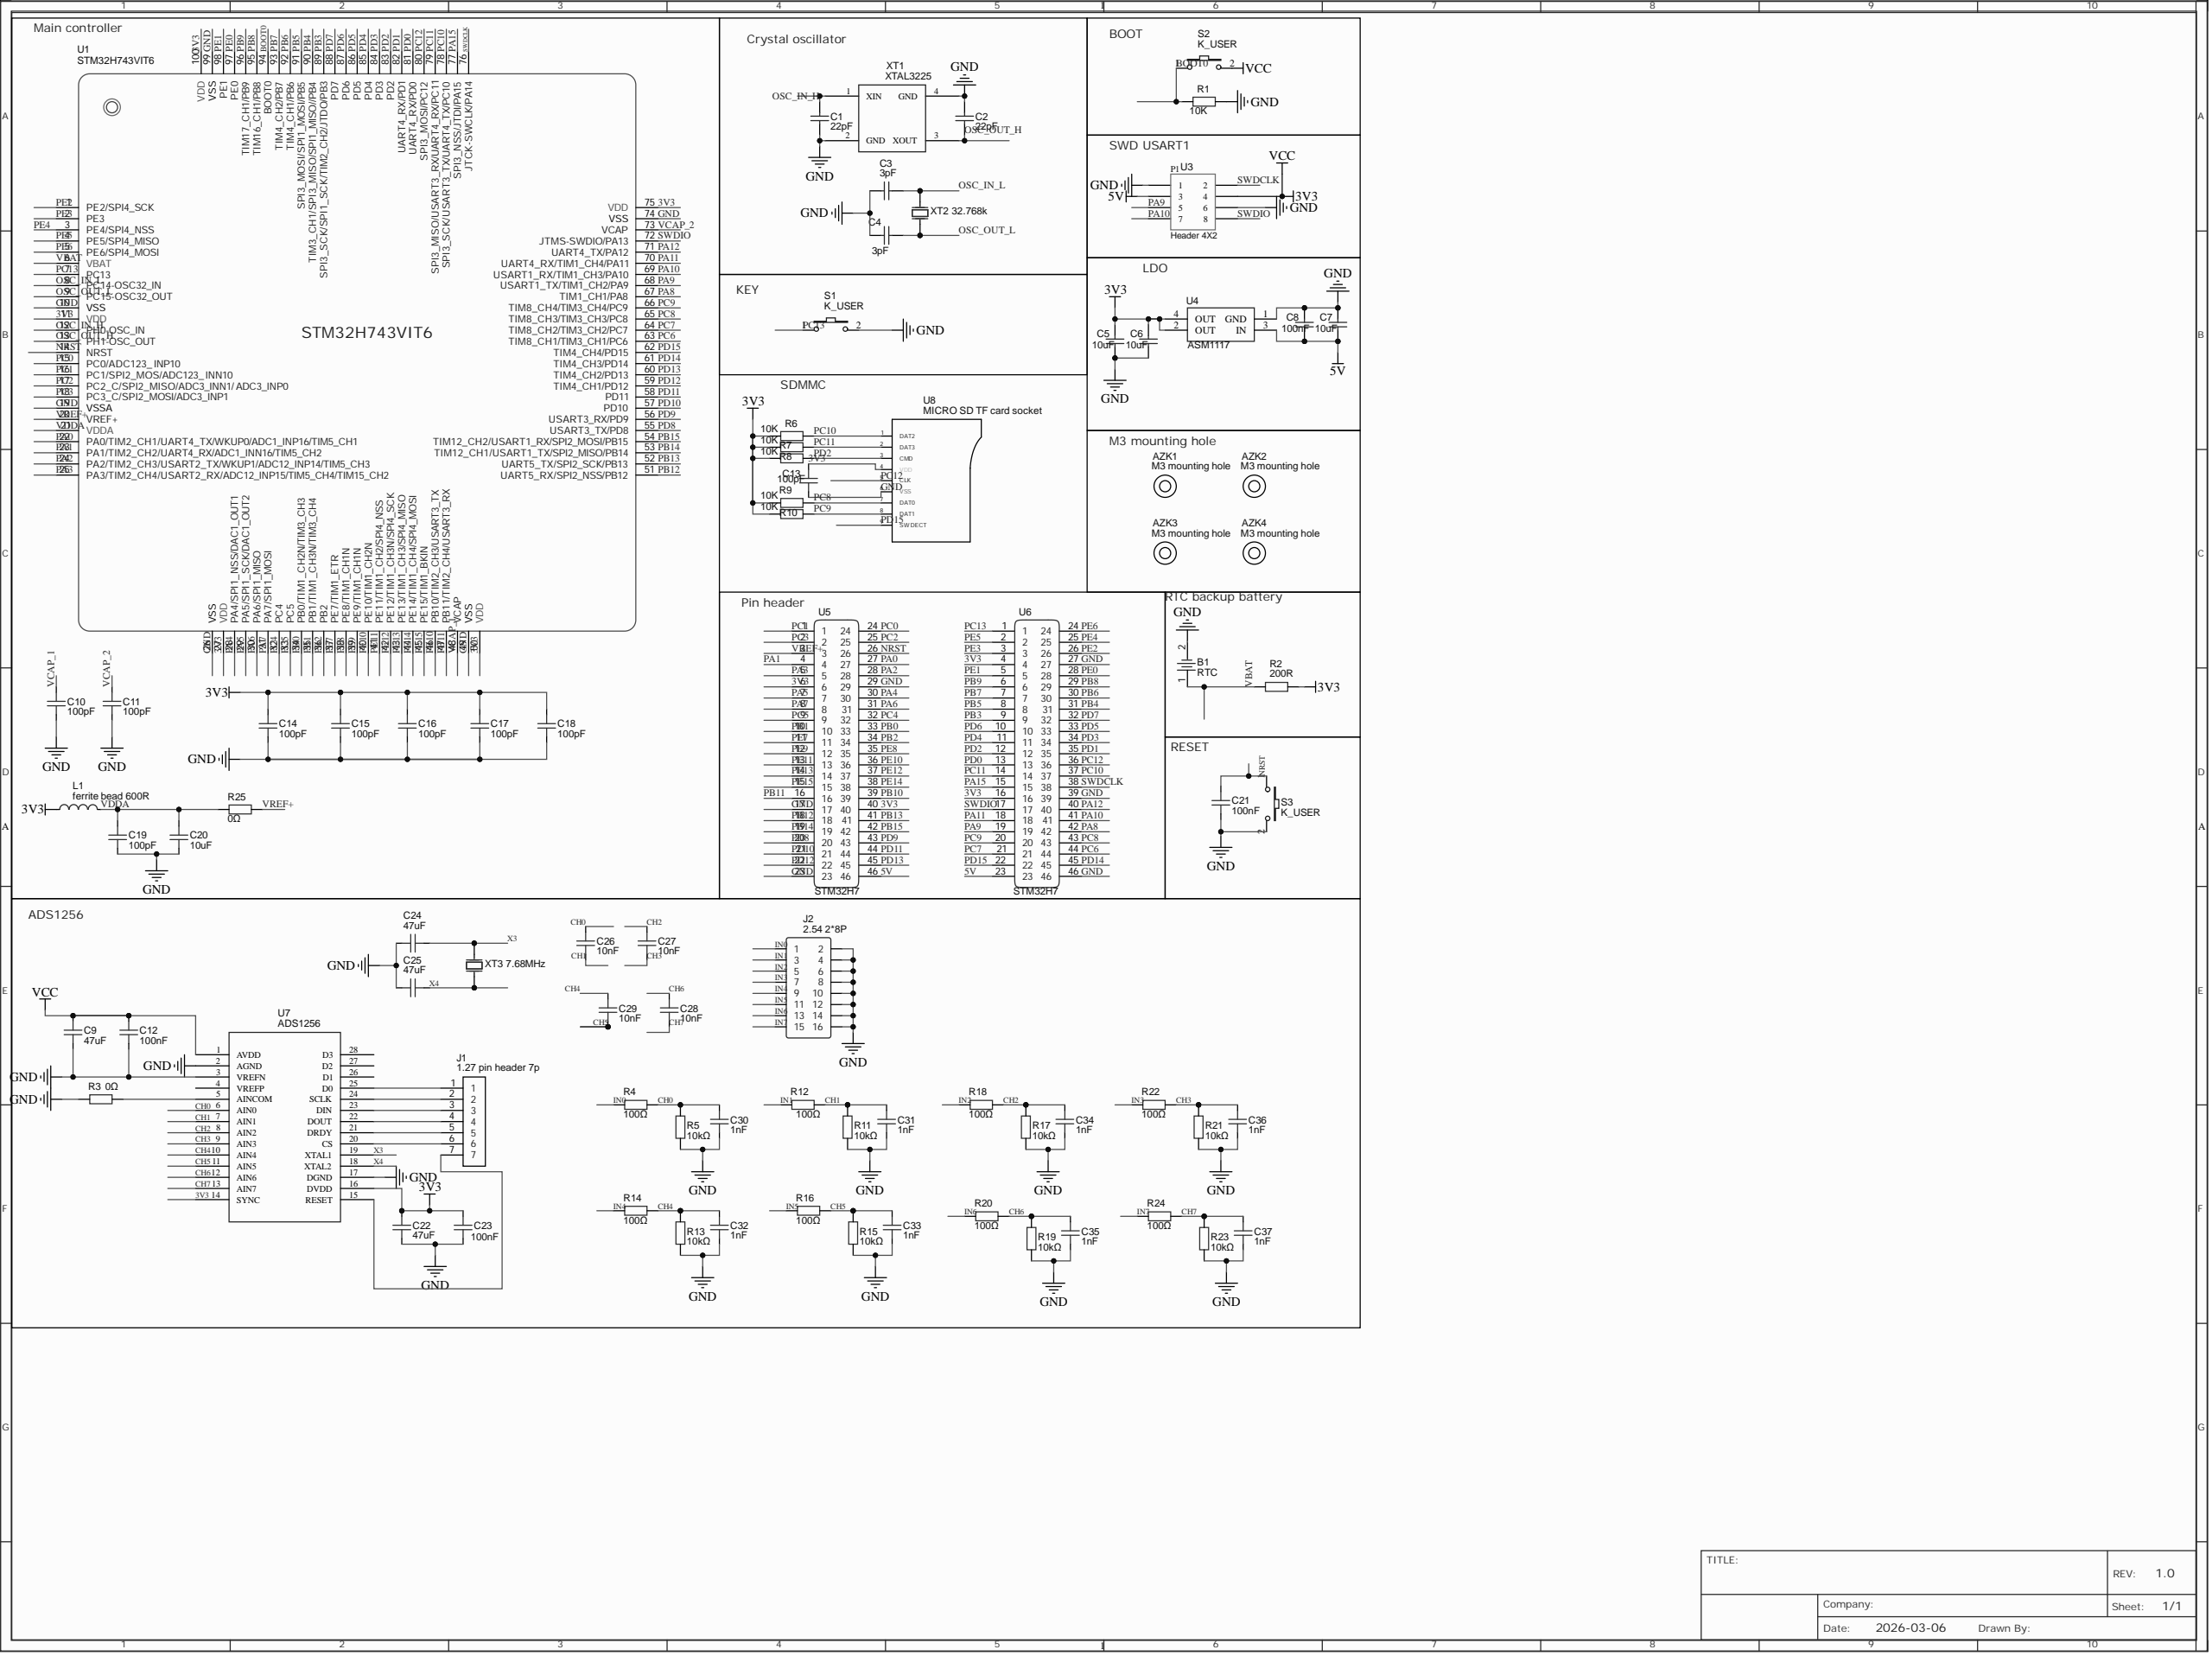Circuit board | Altium Designer | 83 parts | 118 nets
Bill of materials:
Comment,Description,Designator,Footprint,LibRef,Quantity
"M3 mounting hole","","AZK1, AZK2, AZK3, AZK4","M3安装孔(非金属化)","M3安装孔","4"
"RTC","","B1","焊盘引出RTC","RTC","1"
"22pF","","C1, C2","C0402","0402CG220J500NT","2"
"3pF","","C3, C4","C0402","0402CG220J500NT","2"
"10uF","","C5, C6, C7, C20","C0402","0402CG220J500NT, C1005CH2A101K050BA","4"
"100nF","","C8, C12, C21, C23","C0402","0402CG220J500NT, C1005CH2A101K050BA","4"
"47uF","","C9, C22, C24, C25","C0402","C1005CH2A101K050BA","4"
"100pF","","C10, C11, C13, C14, C15, C16, C17, C18, C19","C0402","C1005CH2A101K050BA","9"
"10nF","","C26, C27, C28, C29","C0402","C1005CH2A101K050BA","4"
"1nF","","C30, C31, C32, C33, C34, C35, C36, C37","C0402","C1005CH2A101K050BA","8"
"1.27 pin header 7p","","J1","1.27排针7P","1.27排针7p","1"
"2.54 2*8P","","J2","HDR-TH_16P-P2.54-V-R2-C8-S2.54","2.54mm,2×8Double female header","1"
"ferrite bead 600R","","L1","L0402","SDCL1005C22NJTDF","1"
"10K","","R1, R6, R7, R8, R9, R10","贴片电阻0402封装","RMC080510K1%N","6"
"200R","","R2","贴片电阻0402封装","RMC080510K1%N","1"
"0Ω","","R3, R25","贴片电阻0402封装","RMC080510K1%N","2"
"100Ω","","R4, R12, R14, R16, R18, R20, R22, R24","贴片电阻0402封装","RMC080510K1%N","8"
"10kΩ","","R5, R11, R13, R15, R17, R19, R21, R23","贴片电阻0402封装","RMC080510K1%N","8"
"K_USER","","S1, S2, S3","按键开关4.5","K_USER","3"
"STM32H743VIT6","","U1","STM32H743VIT6","STM32H743VIT6","1"
"HDR_2*4P","","U3","HDR_2*4P","HDR_2*4P","1"
"ASM1117","","U4","AMS1117-SOT-223","ASM1117","1"
"STM32H7","","U5, U6","2*23","2*23","2"
"ADS1256","","U7","SSOP-28_L10.2-W5.3-P0.65-LS7.8-BL","ADS1256","1"
"MICRO SD TF card socket","","U8","MICRO SD TF卡座","MICRO SD TF卡座","1"
"XTAL3225","","XT1","XTAL3225","XTAL3225","1"
"32.768k","","XT2","SMD-2012_2P","SC-20S32.768kHz20PPM9pF","1"
"7.68MHz","","XT3","SMD-2012_2P","SC-20S32.768kHz20PPM9pF","1"
Netlist (Protel format):
[
AZK1
M3安装孔(非金属化)
M3 mounting hole



]
[
AZK2
M3安装孔(非金属化)
M3 mounting hole



]
[
AZK3
M3安装孔(非金属化)
M3 mounting hole



]
[
AZK4
M3安装孔(非金属化)
M3 mounting hole



]
[
B1
焊盘引出RTC
RTC



]
[
C1
C0402
22pF



]
[
C2
C0402
22pF



]
[
C3
C0402
3pF



]
[
C4
C0402
3pF



]
[
C5
C0402
10uF



]
[
C6
C0402
10uF



]
[
C7
C0402
10uF



]
[
C8
C0402
100nF



]
[
C9
C0402
47uF



]
[
C10
C0402
100pF



]
[
C11
C0402
100pF



]
[
C12
C0402
100nF



]
[
C13
C0402
100pF



]
[
C14
C0402
100pF



]
[
C15
C0402
100pF



]
[
C16
C0402
100pF



]
[
C17
C0402
100pF



]
[
C18
C0402
100pF



]
[
C19
C0402
100pF



]
[
C20
C0402
10uF



]
[
C21
C0402
100nF



]
[
C22
C0402
47uF



]
[
C23
C0402
100nF



]
[
C24
C0402
47uF



]
[
C25
C0402
47uF



]
[
C26
C0402
10nF



]
[
C27
C0402
10nF



]
[
C28
C0402
10nF



]
[
C29
C0402
10nF



]
[
C30
C0402
1nF



]
[
C31
C0402
1nF



]
[
C32
C0402
1nF



]
[
C33
C0402
1nF



]
[
C34
C0402
1nF



]
[
C35
C0402
1nF



]
[
C36
C0402
1nF



]
[
C37
C0402
1nF



]
[
J1
1.27排针7P
1.27 pin header 7p



]
[
J2
HDR-TH_16P-P2.54-V-R2-C8-S2.54
2.54 2*8P



]
[
L1
L0402
ferrite bead 600R



]
[
R1
贴片电阻0402封装
10K



]
[
R2
贴片电阻0402封装
200R



]
[
R3
贴片电阻0402封装
0Ω



]
[
R4
贴片电阻0402封装
100Ω



]
[
R5
贴片电阻0402封装
10kΩ



]
[
R6
贴片电阻0402封装
10K



]
[
R7
贴片电阻0402封装
10K



]
[
R8
贴片电阻0402封装
10K



]
[
R9
贴片电阻0402封装
10K



]
[
R10
贴片电阻0402封装
10K



]
[
R11
贴片电阻0402封装
10kΩ



]
[
R12
贴片电阻0402封装
100Ω



]
[
R13
贴片电阻0402封装
10kΩ



]
[
R14
贴片电阻0402封装
100Ω



]
[
R15
贴片电阻0402封装
10kΩ



]
[
R16
贴片电阻0402封装
100Ω



]
[
R17
贴片电阻0402封装
10kΩ



]
[
R18
贴片电阻0402封装
100Ω



]
[
R19
贴片电阻0402封装
10kΩ



]
[
R20
贴片电阻0402封装
100Ω



]
[
R21
贴片电阻0402封装
10kΩ



]
[
R22
贴片电阻0402封装
100Ω



]
[
R23
贴片电阻0402封装
10kΩ



]
[
R24
贴片电阻0402封装
100Ω



]
[
R25
贴片电阻0402封装
0Ω



]
[
S1
按键开关4.5
K_USER



]
[
S2
按键开关4.5
K_USER



]
[
S3
按键开关4.5
K_USER



]
[
U1
STM32H743VIT6
STM32H743VIT6



]
[
U3
HDR_2*4P
HDR_2*4P



]
[
U4
AMS1117-SOT-223
ASM1117



]
[
U5
2*23
STM32H7



]
[
U6
2*23
STM32H7



]
[
U7
SSOP-28_L10.2-W5.3-P0.65-LS7.8-BL
ADS1256



]
[
U8
MICRO SD TF卡座
MICRO SD TF card socket



]
[
XT1
XTAL3225
XTAL3225



]
[
XT2
SMD-2012_2P
32.768k



]
[
XT3
SMD-2012_2P
7.68MHz



]
(
X4
C25-1
U7-18
XT3-2
)
(
X3
C24-1
U7-19
XT3-1
)
(
VREF+
R25-2
U1-20
U5-3
)
(
VDDA
C19-2
C20-2
L1-2
R25-1
U1-21
)
(
VCAP_2
C11-2
U1-73
)
(
VCAP_1
C10-2
U1-48
)
(
VBAT
B1-1
R2-2
U1-6
)
(
SWDIO
U1-72
U3-8
U6-17
)
(
SWDCLK
U1-76
U3-2
U6-38
)
(
PE15
U1-45
U5-15
)
(
PE14
U1-44
U5-38
)
(
PE13
U1-43
U5-14
)
(
PE12
U1-42
U5-37
)
(
PE11
U1-41
U5-13
)
(
PE10
U1-40
U5-36
)
(
PE9
U1-39
U5-12
)
(
PE8
U1-38
U5-35
)
(
PE7
U1-37
U5-11
)
(
PE6
U1-5
U6-24
)
(
PE5
U1-4
U6-2
)
(
PE4
U1-3
U6-25
)
(
PE3
U1-2
U6-3
)
(
PE2
U1-1
U6-26
)
(
PE1
U1-98
U6-5
)
(
PE0
U1-97
U6-28
)
(
PD15
U1-62
U6-22
U8-9
)
(
PD14
U1-61
U6-45
)
(
PD13
U1-60
U5-45
)
(
PD12
U1-59
U5-22
)
(
PD11
U1-58
U5-44
)
(
PD10
U1-57
U5-21
)
(
PD9
U1-56
U5-43
)
(
PD8
U1-55
U5-20
)
(
PD7
U1-88
U6-32
)
(
PD6
U1-87
U6-10
)
(
PD5
U1-86
U6-33
)
(
PD4
U1-85
U6-11
)
(
PD3
U1-84
U6-34
)
(
PD2
R8-2
U1-83
U6-12
U8-3
)
(
PD1
U1-82
U6-35
)
(
PD0
U1-81
U6-13
)
(
PC13
S1-1
U1-7
U6-1
)
(
PC12
U1-80
U6-36
U8-5
)
(
PC11
R7-2
U1-79
U6-14
U8-2
)
(
PC10
R6-2
U1-78
U6-37
U8-1
)
(
PC9
R10-2
U1-66
U6-20
U8-8
)
(
PC8
R9-2
U1-65
U6-43
U8-7
)
(
PC7
U1-64
U6-21
)
(
PC6
U1-63
U6-44
)
(
PC5
U1-33
U5-9
)
(
PC4
U1-32
U5-32
)
(
PC3
U1-18
U5-2
)
(
PC2
U1-17
U5-25
)
(
PC1
U1-16
U5-1
)
(
PC0
U1-15
U5-24
)
(
PB15
U1-54
U5-42
)
(
PB14
U1-53
U5-19
)
(
PB13
U1-52
U5-41
)
(
PB12
U1-51
U5-18
)
(
PB11
U1-47
U5-16
)
(
PB10
U1-46
U5-39
)
(
PB9
U1-96
U6-6
)
(
PB8
U1-95
U6-29
)
(
PB7
U1-93
U6-7
)
(
PB6
U1-92
U6-30
)
(
PB5
U1-91
U6-8
)
(
PB4
U1-90
U6-31
)
(
PB3
U1-89
U6-9
)
(
PB2
U1-36
U5-34
)
(
PB1
U1-35
U5-10
)
(
PB0
U1-34
U5-33
)
(
PA15
U1-77
U6-15
)
(
PA12
U1-71
U6-40
)
(
PA11
U1-70
U6-18
)
(
PA10
U1-69
U3-7
U6-41
)
(
PA9
U1-68
U3-5
U6-19
)
(
PA8
U1-67
U6-42
)
(
PA7
U1-31
U5-8
)
(
PA6
U1-30
U5-31
)
(
PA5
U1-29
U5-7
)
(
PA4
U1-28
U5-30
)
(
PA3
U1-25
U5-5
)
(
PA2
U1-24
U5-28
)
(
PA1
U1-23
U5-4
)
(
PA0
U1-22
U5-27
)
(
OSC_OUT_L
C4-1
U1-9
XT2-2
)
(
OSC_OUT_H
C2-1
U1-13
XT1-3
)
(
OSC_IN_L
C3-1
U1-8
XT2-1
)
(
OSC_IN_H
C1-2
U1-12
XT1-1
)
(
NRST
C21-2
S3-1
U1-14
U5-26
)
(
NetR3_2
R3-2
U7-5
)
(
NetJ1_7
J1-7
U7-15
)
(
NetJ1_6
J1-6
U7-20
)
(
NetJ1_5
J1-5
U7-21
)
(
NetJ1_4
J1-4
U7-22
)
(
NetJ1_3
J1-3
U7-23
)
(
NetJ1_2
J1-2
U7-24
)
(
NetJ1_1
J1-1
U7-25
)
(
IN7
J2-15
R24-1
)
(
IN6
J2-13
R20-1
)
(
IN5
J2-11
R16-1
)
(
IN4
J2-9
R14-1
)
(
IN3
J2-7
R22-1
)
(
IN2
J2-5
R18-1
)
(
IN1
J2-3
R12-1
)
(
IN0
J2-1
R4-1
)
(
GND
B1-2
C1-1
C2-2
C3-2
C4-2
C5-1
C6-1
C7-2
C8-2
C9-1
C10-1
C11-1
C12-1
C13-1
C14-1
C15-1
C16-1
C17-1
C18-1
C19-1
C20-1
C21-1
C22-1
C23-1
C24-2
C25-2
C30-2
C31-2
C32-2
C33-2
C34-2
C35-2
C36-2
C37-2
J2-2
J2-4
J2-6
J2-8
J2-10
J2-12
J2-14
J2-16
R1-2
R3-1
R5-1
R11-1
R13-1
R15-1
R17-1
R19-1
R21-1
R23-1
S1-2
S3-2
U1-10
U1-19
U1-26
U1-49
U1-74
U1-99
U3-1
U3-6
U4-1
U5-17
U5-23
U5-29
U6-27
U6-39
U6-46
U7-2
U7-3
U7-17
U8-6
XT1-2
XT1-4
)
(
CH7
C28-2
C37-1
R23-2
R24-2
U7-13
)
(
CH6
C28-1
C35-1
R19-2
R20-2
U7-12
)
(
CH5
C29-2
C33-1
R15-2
R16-2
U7-11
)
(
CH4
C29-1
C32-1
R13-2
R14-2
U7-10
)
(
CH3
C27-2
C36-1
R21-2
R22-2
U7-9
)
(
CH2
C27-1
C34-1
R17-2
R18-2
U7-8
)
(
CH1
C26-2
C31-1
R11-2
R12-2
U7-7
)
(
CH0
C26-1
C30-1
R4-2
R5-2
U7-6
)
(
BOOT0
R1-1
S2-1
U1-94
)
(
5V
C7-1
C8-1
U3-3
U4-3
U5-46
U6-23
)
(
3V3
C5-2
C6-2
C9-2
C12-2
C13-2
C14-2
C15-2
C16-2
C17-2
C18-2
C22-2
C23-2
L1-1
R2-1
R6-1
R7-1
R8-1
R9-1
R10-1
S2-2
U1-11
U1-27
U1-50
U1-75
U1-100
U3-4
U4-2
U4-4
U5-6
U5-40
U6-4
U6-16
U7-1
U7-14
U7-16
U8-4
)